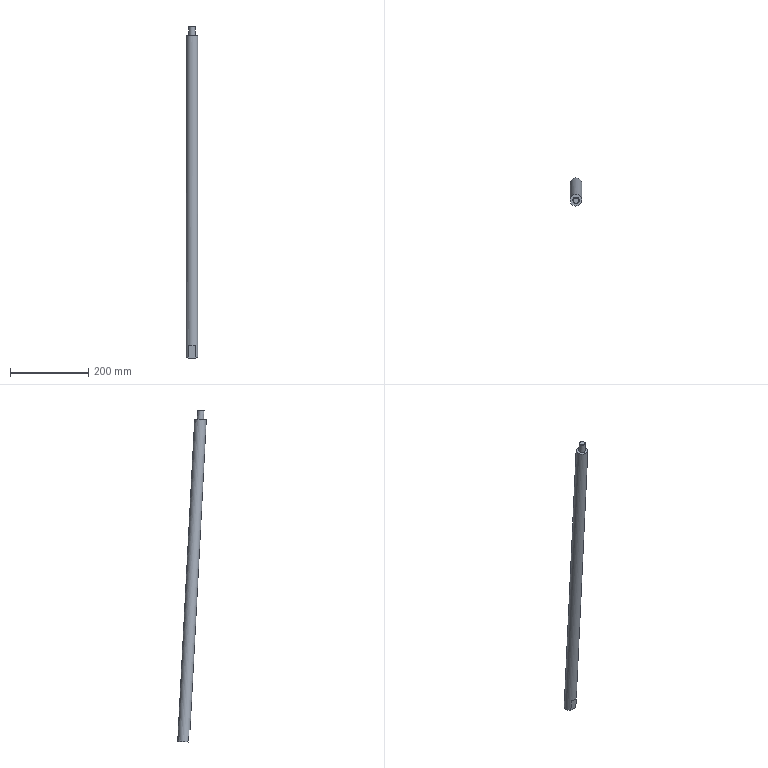Part | STEP file | solid 221 | 1 solid | 11 faces | box 30 x 73.163 x 849.352 mm | volume 585466 mm3 | plane 5 | cylinder 3 | cone 3 | commonest cylinder face diameters 10.2 x1 16 x1 30 x1